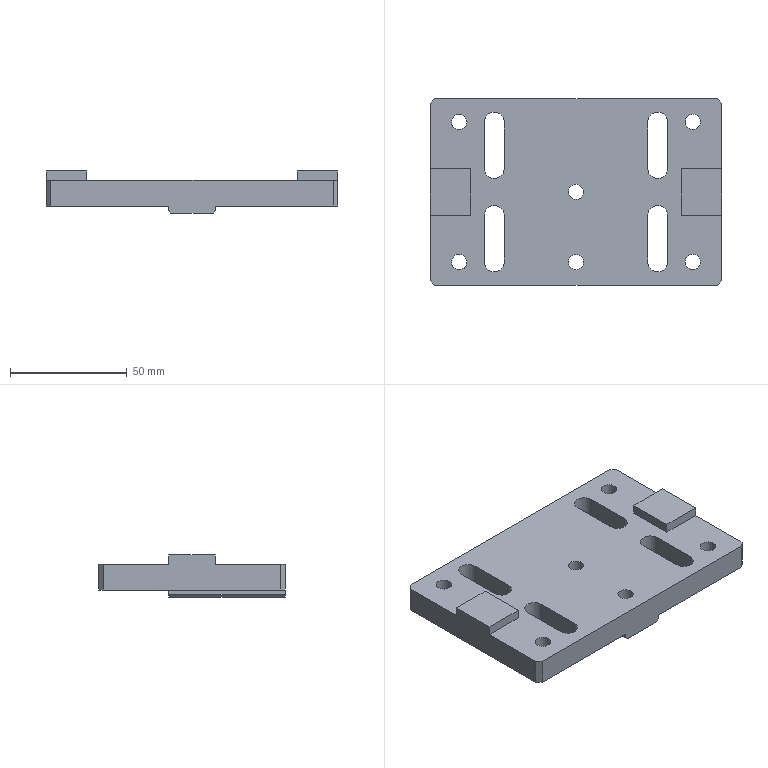NC program | NX | posted with a generic post | part box 125 x 80 x 18 mm
Lines 3321 to 3483 of 3483:
(PLANAR_MILL_COPY , TOOL : D8A45)
N6592 T06 M6
N6594 G54
N6596 G17 G0 G90 X12.1 Y16.501 S7000 M3
N6598 G43 Z30. H6
N6600 Z0.
N6602 G94 G1 Z-1.5 F1250.
N6604 X11. Y15.866
N6606 G3 X10.5 Y15. R1.
N6608 G1 Y-10.
N6610 G2 X9. Y-11.5 R1.5
N6612 G1 X-9.
N6614 G2 X-10.5 Y-10. R1.5
N6616 G1 Y40.
N6618 G2 X-9. Y41.5 R1.5
N6620 G1 X9.
N6622 G2 X10.5 Y40. R1.5
N6624 G1 Y15.
N6626 G3 X11. Y14.134 R1.
N6628 G1 X12.1 Y13.499
N6630 Z0.
N6632 G0 Z30.
(PLANAR_MILL_COPY_COPY , TOOL : D8A45)
N6634 X49.415 Y-32.431
N6636 Z-3.
N6638 G1 Z-4.5
N6640 X49.134 Y-33.6
N6642 G3 X50. Y-34.1 R1.
N6644 X54.1 Y-30. R4.1
N6646 X50. Y-34.1 R-4.1
N6648 X50.866 Y-33.6 R1.
N6650 G1 X50.585 Y-32.431
N6652 Z-3.
N6654 G0 Z30.
N6656 X36.25 Y-21.501
N6658 Z-3.
N6660 G1 Z-4.5
N6662 X37.35 Y-20.866
N6664 G3 X37.85 Y-20. R1.
N6666 G1 Y-10.
N6668 G3 X35. Y-7.15 R2.85
N6670 X32.15 Y-10. R2.85
N6672 G1 Y-30.
N6674 G3 X35. Y-32.85 R2.85
N6676 X37.85 Y-30. R2.85
N6678 G1 Y-20.
N6680 G3 X37.35 Y-19.134 R1.
N6682 G1 X36.25 Y-18.499
N6684 Z-3.
N6686 G0 Z30.
N6688 X50.585 Y32.431
N6690 Z-3.
N6692 G1 Z-4.5
N6694 X50.866 Y33.6
N6696 G3 X50. Y34.1 R1.
N6698 X45.9 Y30. R4.1
N6700 X50. Y34.1 R-4.1
N6702 X49.134 Y33.6 R1.
N6704 G1 X49.415 Y32.431
N6706 Z-3.
N6708 G0 Z30.
N6710 X36.25 Y18.499
N6712 Z-3.
N6714 G1 Z-4.5
N6716 X37.35 Y19.134
N6718 G3 X37.85 Y20. R1.
N6720 G1 Y30.
N6722 G3 X35. Y32.85 R2.85
N6724 X32.15 Y30. R2.85
N6726 G1 Y10.
N6728 G3 X35. Y7.15 R2.85
N6730 X37.85 Y10. R2.85
N6732 G1 Y20.
N6734 G3 X37.35 Y20.866 R1.
N6736 G1 X36.25 Y21.501
N6738 Z-3.
N6740 G0 Z30.
N6742 X15.204 Y43.183
N6744 Z-3.
N6746 G1 Z-4.5
N6748 X14.482 Y42.379
N6750 G3 X14.277 Y41.4 R1.
N6752 G1 X60.459
N6754 G2 X61.519 Y40.961 R1.5
N6756 G1 X63.461 Y39.019
N6758 G2 X63.9 Y37.959 R1.5
N6760 G1 Y-37.959
N6762 G2 X63.461 Y-39.019 R1.5
N6764 G1 X61.519 Y-40.961
N6766 G2 X60.459 Y-41.4 R1.5
N6768 G1 X-60.459
N6770 G2 X-61.519 Y-40.961 R1.5
N6772 G1 X-63.461 Y-39.019
N6774 G2 X-63.9 Y-37.959 R1.5
N6776 G1 Y37.959
N6778 G2 X-63.461 Y39.019 R1.5
N6780 G1 X-61.519 Y40.961
N6782 G2 X-60.459 Y41.4 R1.5
N6784 G1 X-14.277
N6786 G3 X-14.482 Y42.379 R1.
N6788 G1 X-15.204 Y43.183
N6790 Z-3.
N6792 G0 Z30.
N6794 X-36.25 Y21.501
N6796 Z-3.
N6798 G1 Z-4.5
N6800 X-37.35 Y20.866
N6802 G3 X-37.85 Y20. R1.
N6804 G1 Y10.
N6806 G3 X-35. Y7.15 R2.85
N6808 X-32.15 Y10. R2.85
N6810 G1 Y30.
N6812 G3 X-35. Y32.85 R2.85
N6814 X-37.85 Y30. R2.85
N6816 G1 Y20.
N6818 G3 X-37.35 Y19.134 R1.
N6820 G1 X-36.25 Y18.499
N6822 Z-3.
N6824 G0 Z30.
N6826 X-49.415 Y32.431
N6828 Z-3.
N6830 G1 Z-4.5
N6832 X-49.134 Y33.6
N6834 G3 X-50. Y34.1 R1.
N6836 X-54.1 Y30. R4.1
N6838 X-50. Y34.1 R-4.1
N6840 X-50.866 Y33.6 R1.
N6842 G1 X-50.585 Y32.431
N6844 Z-3.
N6846 G0 Z30.
N6848 X-33.75 Y-21.501
N6850 Z-3.
N6852 G1 Z-4.5
N6854 X-32.65 Y-20.866
N6856 G3 X-32.15 Y-20. R1.
N6858 G1 Y-10.
N6860 G3 X-35. Y-7.15 R2.85
N6862 X-37.85 Y-10. R2.85
N6864 G1 Y-30.
N6866 G3 X-35. Y-32.85 R2.85
N6868 X-32.15 Y-30. R2.85
N6870 G1 Y-20.
N6872 G3 X-32.65 Y-19.134 R1.
N6874 G1 X-33.75 Y-18.499
N6876 Z-3.
N6878 G0 Z30.
N6880 X-50.585 Y-32.431
N6882 Z-3.
N6884 G1 Z-4.5
N6886 X-50.866 Y-33.6
N6888 G3 X-50. Y-34.1 R1.
N6890 X-45.9 Y-30. R4.1
N6892 X-50. Y-34.1 R-4.1
N6894 X-49.134 Y-33.6 R1.
N6896 G1 X-49.415 Y-32.431
N6898 Z-3.
N6900 G0 Z30.
N6902 M5
N6904 M2